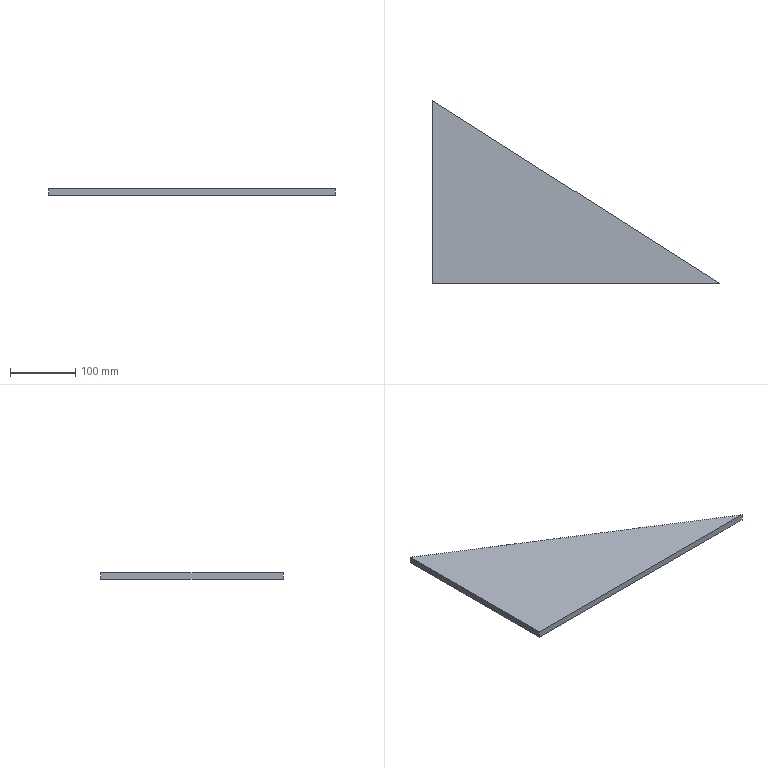Part | SolidWorks | features Extrusion 1 | 1 solid | 5 faces | box 440 x 280 x 10 mm | volume 616000 mm3 | plane 5
STEP:
#1=CARTESIAN_POINT('',(0.,0.,0.));
#2=VERTEX_POINT('',#1);
#3=CARTESIAN_POINT('',(440.,0.,0.));
#4=VERTEX_POINT('',#3);
#5=CARTESIAN_POINT('',(440.,0.,0.));
#6=DIRECTION('',(1.,0.,0.));
#7=VECTOR('',#6,1000.);
#8=LINE('',#5,#7);
#9=EDGE_CURVE('',#2,#4,#8,.T.);
#10=ORIENTED_EDGE('',*,*,#9,.T.);
#11=CARTESIAN_POINT('',(440.,0.,10.));
#12=VERTEX_POINT('',#11);
#13=CARTESIAN_POINT('',(440.,0.,10.));
#14=DIRECTION('',(0.,0.,-1.));
#15=VECTOR('',#14,1000.);
#16=LINE('',#13,#15);
#17=EDGE_CURVE('',#12,#4,#16,.T.);
#18=ORIENTED_EDGE('',*,*,#17,.F.);
#19=CARTESIAN_POINT('',(0.,0.,10.));
#20=VERTEX_POINT('',#19);
#21=CARTESIAN_POINT('',(440.,0.,10.));
#22=DIRECTION('',(1.,0.,0.));
#23=VECTOR('',#22,1000.);
#24=LINE('',#21,#23);
#25=EDGE_CURVE('',#20,#12,#24,.T.);
#26=ORIENTED_EDGE('',*,*,#25,.F.);
#27=CARTESIAN_POINT('',(0.,0.,10.));
#28=DIRECTION('',(0.,0.,-1.));
#29=VECTOR('',#28,1000.);
#30=LINE('',#27,#29);
#31=EDGE_CURVE('',#20,#2,#30,.T.);
#32=ORIENTED_EDGE('',*,*,#31,.T.);
#33=EDGE_LOOP('',(#10,#18,#26,#32));
#34=FACE_OUTER_BOUND('',#33,.T.);
#35=CARTESIAN_POINT('',(440.,0.,10.));
#36=DIRECTION('',(0.,1.,0.));
#37=DIRECTION('',(-1.,0.,0.));
#38=AXIS2_PLACEMENT_3D('',#35,#36,#37);
#39=PLANE('',#38);
#40=ADVANCED_FACE('',(#34),#39,.F.);
#41=CARTESIAN_POINT('',(0.,280.,0.));
#42=VERTEX_POINT('',#41);
#43=CARTESIAN_POINT('',(0.,280.,0.));
#44=DIRECTION('',(-0.8437,0.5369,0.));
#45=VECTOR('',#44,1000.);
#46=LINE('',#43,#45);
#47=EDGE_CURVE('',#4,#42,#46,.T.);
#48=ORIENTED_EDGE('',*,*,#47,.T.);
#49=CARTESIAN_POINT('',(0.,280.,10.));
#50=VERTEX_POINT('',#49);
#51=CARTESIAN_POINT('',(0.,280.,10.));
#52=DIRECTION('',(0.,0.,-1.));
#53=VECTOR('',#52,1000.);
#54=LINE('',#51,#53);
#55=EDGE_CURVE('',#50,#42,#54,.T.);
#56=ORIENTED_EDGE('',*,*,#55,.F.);
#57=CARTESIAN_POINT('',(0.,280.,10.));
#58=DIRECTION('',(-0.8437,0.5369,0.));
#59=VECTOR('',#58,1000.);
#60=LINE('',#57,#59);
#61=EDGE_CURVE('',#12,#50,#60,.T.);
#62=ORIENTED_EDGE('',*,*,#61,.F.);
#63=ORIENTED_EDGE('',*,*,#17,.T.);
#64=EDGE_LOOP('',(#48,#56,#62,#63));
#65=FACE_OUTER_BOUND('',#64,.T.);
#66=CARTESIAN_POINT('',(0.,280.,10.));
#67=DIRECTION('',(-0.5369,-0.8437,0.));
#68=DIRECTION('',(0.8437,-0.5369,0.));
#69=AXIS2_PLACEMENT_3D('',#66,#67,#68);
#70=PLANE('',#69);
#71=ADVANCED_FACE('',(#65),#70,.F.);
#72=CARTESIAN_POINT('',(0.,0.,0.));
#73=DIRECTION('',(0.,-1.,0.));
#74=VECTOR('',#73,1000.);
#75=LINE('',#72,#74);
#76=EDGE_CURVE('',#42,#2,#75,.T.);
#77=ORIENTED_EDGE('',*,*,#76,.T.);
#78=ORIENTED_EDGE('',*,*,#31,.F.);
#79=CARTESIAN_POINT('',(0.,0.,10.));
#80=DIRECTION('',(0.,-1.,0.));
#81=VECTOR('',#80,1000.);
#82=LINE('',#79,#81);
#83=EDGE_CURVE('',#50,#20,#82,.T.);
#84=ORIENTED_EDGE('',*,*,#83,.F.);
#85=ORIENTED_EDGE('',*,*,#55,.T.);
#86=EDGE_LOOP('',(#77,#78,#84,#85));
#87=FACE_OUTER_BOUND('',#86,.T.);
#88=CARTESIAN_POINT('',(0.,0.,10.));
#89=DIRECTION('',(1.,0.,0.));
#90=DIRECTION('',(0.,0.,-1.));
#91=AXIS2_PLACEMENT_3D('',#88,#89,#90);
#92=PLANE('',#91);
#93=ADVANCED_FACE('',(#87),#92,.F.);
#94=ORIENTED_EDGE('',*,*,#25,.T.);
#95=ORIENTED_EDGE('',*,*,#61,.T.);
#96=ORIENTED_EDGE('',*,*,#83,.T.);
#97=EDGE_LOOP('',(#94,#95,#96));
#98=FACE_OUTER_BOUND('',#97,.T.);
#99=CARTESIAN_POINT('',(0.,0.,10.));
#100=DIRECTION('',(0.,0.,-1.));
#101=DIRECTION('',(-1.,0.,0.));
#102=AXIS2_PLACEMENT_3D('',#99,#100,#101);
#103=PLANE('',#102);
#104=ADVANCED_FACE('',(#98),#103,.F.);
#105=ORIENTED_EDGE('',*,*,#9,.F.);
#106=ORIENTED_EDGE('',*,*,#76,.F.);
#107=ORIENTED_EDGE('',*,*,#47,.F.);
#108=EDGE_LOOP('',(#105,#106,#107));
#109=FACE_OUTER_BOUND('',#108,.T.);
#110=CARTESIAN_POINT('',(0.,0.,0.));
#111=DIRECTION('',(0.,0.,-1.));
#112=DIRECTION('',(-1.,0.,0.));
#113=AXIS2_PLACEMENT_3D('',#110,#111,#112);
#114=PLANE('',#113);
#115=ADVANCED_FACE('',(#109),#114,.T.);
#116=CLOSED_SHELL('',(#40,#71,#93,#104,#115));
#117=MANIFOLD_SOLID_BREP('',#116);
#118=CARTESIAN_POINT('',(0.,0.,0.));
#119=DIRECTION('',(0.,0.,1.));
#120=DIRECTION('',(1.,0.,0.));
#121=AXIS2_PLACEMENT_3D('',#118,#119,#120);
#122=(LENGTH_UNIT()NAMED_UNIT(*)SI_UNIT(.MILLI.,.METRE.));
#123=UNCERTAINTY_MEASURE_WITH_UNIT(LENGTH_MEASURE(0.00001),#122,'','');
#124=(NAMED_UNIT(*)PLANE_ANGLE_UNIT()SI_UNIT($,.RADIAN.));
#125=(NAMED_UNIT(*)SI_UNIT($,.STERADIAN.)SOLID_ANGLE_UNIT());
#126=(GEOMETRIC_REPRESENTATION_CONTEXT(3)GLOBAL_UNCERTAINTY_ASSIGNED_CONTEXT((#123))GLOBAL_UNIT_ASSIGNED_CONTEXT((#122,#124,#125))REPRESENTATION_CONTEXT('',''));
#127=ADVANCED_BREP_SHAPE_REPRESENTATION('',(#117,#121),#126);